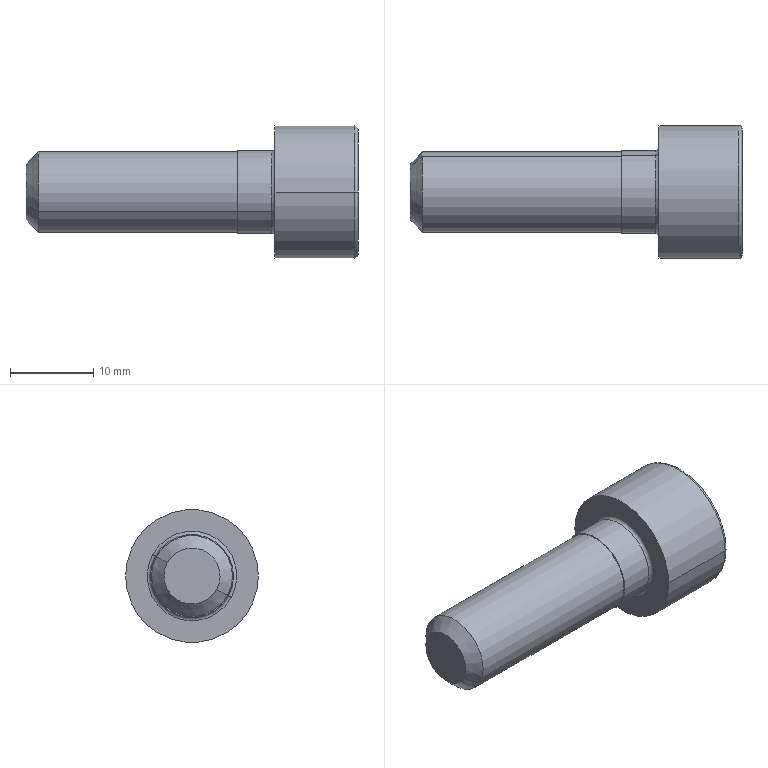Part | NX | features BREP 1 | 1 solid | 31 faces | box 40 x 16 x 16 mm | volume 3905 mm3 | cylinder 12 | plane 11 | torus 4 | cone 4 | commonest cylinder face diameters 9.149 x6 9.756 x2 10 x2 16 x2
STEP:
#1=CARTESIAN_POINT('',(0.,-8.,0.));
#2=VERTEX_POINT('',#1);
#3=CARTESIAN_POINT('',(0.,8.,0.));
#4=VERTEX_POINT('',#3);
#5=CARTESIAN_POINT('',(0.,0.,0.));
#6=DIRECTION('',(-1.,0.,0.));
#7=DIRECTION('',(0.,-1.,0.));
#8=AXIS2_PLACEMENT_3D('',#5,#6,#7);
#9=CIRCLE('',#8,8.);
#10=EDGE_CURVE('',#2,#4,#9,.T.);
#11=ORIENTED_EDGE('',*,*,#10,.F.);
#12=CARTESIAN_POINT('',(9.6,-8.,0.));
#13=VERTEX_POINT('',#12);
#14=CARTESIAN_POINT('',(9.6,-8.,0.));
#15=DIRECTION('',(-1.,0.,0.));
#16=VECTOR('',#15,1000.);
#17=LINE('',#14,#16);
#18=EDGE_CURVE('',#13,#2,#17,.T.);
#19=ORIENTED_EDGE('',*,*,#18,.F.);
#20=CARTESIAN_POINT('',(9.6,8.,0.));
#21=VERTEX_POINT('',#20);
#22=CARTESIAN_POINT('',(9.6,0.,0.));
#23=DIRECTION('',(1.,0.,0.));
#24=DIRECTION('',(0.,1.,0.));
#25=AXIS2_PLACEMENT_3D('',#22,#23,#24);
#26=CIRCLE('',#25,8.);
#27=EDGE_CURVE('',#21,#13,#26,.T.);
#28=ORIENTED_EDGE('',*,*,#27,.F.);
#29=CARTESIAN_POINT('',(9.6,8.,0.));
#30=DIRECTION('',(-1.,0.,0.));
#31=VECTOR('',#30,1000.);
#32=LINE('',#29,#31);
#33=EDGE_CURVE('',#21,#4,#32,.T.);
#34=ORIENTED_EDGE('',*,*,#33,.T.);
#35=EDGE_LOOP('',(#11,#19,#28,#34));
#36=FACE_BOUND('',#35,.T.);
#37=CARTESIAN_POINT('',(5.,0.,0.));
#38=DIRECTION('',(1.,0.,0.));
#39=DIRECTION('',(0.,1.,0.));
#40=AXIS2_PLACEMENT_3D('',#37,#38,#39);
#41=CYLINDRICAL_SURFACE('',#40,8.);
#42=ADVANCED_FACE('',(#36),#41,.T.);
#43=CARTESIAN_POINT('',(0.,0.,0.));
#44=DIRECTION('',(-1.,0.,0.));
#45=DIRECTION('',(0.,1.,0.));
#46=AXIS2_PLACEMENT_3D('',#43,#44,#45);
#47=CIRCLE('',#46,8.);
#48=EDGE_CURVE('',#4,#2,#47,.T.);
#49=ORIENTED_EDGE('',*,*,#48,.F.);
#50=ORIENTED_EDGE('',*,*,#33,.F.);
#51=CARTESIAN_POINT('',(9.6,0.,0.));
#52=DIRECTION('',(-1.,0.,0.));
#53=DIRECTION('',(0.,1.,0.));
#54=AXIS2_PLACEMENT_3D('',#51,#52,#53);
#55=CIRCLE('',#54,8.);
#56=EDGE_CURVE('',#21,#13,#55,.T.);
#57=ORIENTED_EDGE('',*,*,#56,.T.);
#58=ORIENTED_EDGE('',*,*,#18,.T.);
#59=EDGE_LOOP('',(#49,#50,#57,#58));
#60=FACE_BOUND('',#59,.T.);
#61=CARTESIAN_POINT('',(5.,0.,0.));
#62=DIRECTION('',(1.,0.,0.));
#63=DIRECTION('',(0.,1.,0.));
#64=AXIS2_PLACEMENT_3D('',#61,#62,#63);
#65=CYLINDRICAL_SURFACE('',#64,8.);
#66=ADVANCED_FACE('',(#60),#65,.T.);
#67=ORIENTED_EDGE('',*,*,#56,.F.);
#68=CARTESIAN_POINT('',(10.,7.6,0.));
#69=VERTEX_POINT('',#68);
#70=CARTESIAN_POINT('',(9.6,7.6,0.));
#71=DIRECTION('',(0.,0.,-1.));
#72=DIRECTION('',(0.,1.,0.));
#73=AXIS2_PLACEMENT_3D('',#70,#71,#72);
#74=CIRCLE('',#73,0.4);
#75=EDGE_CURVE('',#69,#21,#74,.F.);
#76=ORIENTED_EDGE('',*,*,#75,.F.);
#77=CARTESIAN_POINT('',(10.,-7.6,0.));
#78=VERTEX_POINT('',#77);
#79=CARTESIAN_POINT('',(10.,0.,0.));
#80=DIRECTION('',(1.,0.,0.));
#81=DIRECTION('',(0.,0.8749,-0.4843));
#82=AXIS2_PLACEMENT_3D('',#79,#80,#81);
#83=CIRCLE('',#82,7.6);
#84=EDGE_CURVE('',#78,#69,#83,.T.);
#85=ORIENTED_EDGE('',*,*,#84,.F.);
#86=CARTESIAN_POINT('',(9.6,-7.6,0.));
#87=DIRECTION('',(0.,0.,1.));
#88=DIRECTION('',(0.,-1.,0.));
#89=AXIS2_PLACEMENT_3D('',#86,#87,#88);
#90=CIRCLE('',#89,0.4);
#91=EDGE_CURVE('',#78,#13,#90,.F.);
#92=ORIENTED_EDGE('',*,*,#91,.T.);
#93=EDGE_LOOP('',(#67,#76,#85,#92));
#94=FACE_BOUND('',#93,.T.);
#95=CARTESIAN_POINT('',(9.6,0.,0.));
#96=DIRECTION('',(1.,0.,0.));
#97=DIRECTION('',(0.,-0.8749,0.4843));
#98=AXIS2_PLACEMENT_3D('',#95,#96,#97);
#99=TOROIDAL_SURFACE('',#98,7.6,0.4);
#100=ADVANCED_FACE('',(#94),#99,.T.);
#101=ORIENTED_EDGE('',*,*,#27,.T.);
#102=ORIENTED_EDGE('',*,*,#91,.F.);
#103=CARTESIAN_POINT('',(10.,0.,0.));
#104=DIRECTION('',(1.,0.,0.));
#105=DIRECTION('',(0.,1.,0.));
#106=AXIS2_PLACEMENT_3D('',#103,#104,#105);
#107=CIRCLE('',#106,7.6);
#108=EDGE_CURVE('',#69,#78,#107,.T.);
#109=ORIENTED_EDGE('',*,*,#108,.F.);
#110=ORIENTED_EDGE('',*,*,#75,.T.);
#111=EDGE_LOOP('',(#101,#102,#109,#110));
#112=FACE_BOUND('',#111,.T.);
#113=CARTESIAN_POINT('',(9.6,0.,0.));
#114=DIRECTION('',(1.,0.,0.));
#115=DIRECTION('',(0.,1.,0.));
#116=AXIS2_PLACEMENT_3D('',#113,#114,#115);
#117=TOROIDAL_SURFACE('',#116,7.6,0.4);
#118=ADVANCED_FACE('',(#112),#117,.T.);
#119=ORIENTED_EDGE('',*,*,#84,.T.);
#120=ORIENTED_EDGE('',*,*,#108,.T.);
#121=EDGE_LOOP('',(#119,#120));
#122=FACE_BOUND('',#121,.T.);
#123=CARTESIAN_POINT('',(10.,4.,-2.219));
#124=VERTEX_POINT('',#123);
#125=CARTESIAN_POINT('',(10.,3.922,-2.354));
#126=VERTEX_POINT('',#125);
#127=CARTESIAN_POINT('',(10.,0.,0.));
#128=DIRECTION('',(-1.,0.,0.));
#129=DIRECTION('',(0.,0.8744,-0.4852));
#130=AXIS2_PLACEMENT_3D('',#127,#128,#129);
#131=CIRCLE('',#130,4.574);
#132=EDGE_CURVE('',#124,#126,#131,.T.);
#133=ORIENTED_EDGE('',*,*,#132,.T.);
#134=CARTESIAN_POINT('',(10.,0.07788,-4.574));
#135=VERTEX_POINT('',#134);
#136=CARTESIAN_POINT('',(10.,3.922,-2.354));
#137=DIRECTION('',(0.,-0.866,-0.5));
#138=VECTOR('',#137,1000.);
#139=LINE('',#136,#138);
#140=EDGE_CURVE('',#126,#135,#139,.T.);
#141=ORIENTED_EDGE('',*,*,#140,.T.);
#142=CARTESIAN_POINT('',(10.,-0.07788,-4.574));
#143=VERTEX_POINT('',#142);
#144=CARTESIAN_POINT('',(10.,0.,0.));
#145=DIRECTION('',(1.,0.,0.));
#146=DIRECTION('',(0.,-0.01703,-0.9999));
#147=AXIS2_PLACEMENT_3D('',#144,#145,#146);
#148=CIRCLE('',#147,4.574);
#149=EDGE_CURVE('',#143,#135,#148,.T.);
#150=ORIENTED_EDGE('',*,*,#149,.F.);
#151=CARTESIAN_POINT('',(10.,-3.922,-2.354));
#152=VERTEX_POINT('',#151);
#153=CARTESIAN_POINT('',(10.,-0.07788,-4.574));
#154=DIRECTION('',(0.,-0.866,0.5));
#155=VECTOR('',#154,1000.);
#156=LINE('',#153,#155);
#157=EDGE_CURVE('',#143,#152,#156,.T.);
#158=ORIENTED_EDGE('',*,*,#157,.T.);
#159=CARTESIAN_POINT('',(10.,-4.,-2.219));
#160=VERTEX_POINT('',#159);
#161=CARTESIAN_POINT('',(10.,0.,0.));
#162=DIRECTION('',(-1.,0.,0.));
#163=DIRECTION('',(0.,-0.8574,-0.5147));
#164=AXIS2_PLACEMENT_3D('',#161,#162,#163);
#165=CIRCLE('',#164,4.574);
#166=EDGE_CURVE('',#152,#160,#165,.T.);
#167=ORIENTED_EDGE('',*,*,#166,.T.);
#168=CARTESIAN_POINT('',(10.,-4.,2.219));
#169=VERTEX_POINT('',#168);
#170=CARTESIAN_POINT('',(10.,-4.,-2.219));
#171=DIRECTION('',(0.,0.,1.));
#172=VECTOR('',#171,1000.);
#173=LINE('',#170,#172);
#174=EDGE_CURVE('',#160,#169,#173,.T.);
#175=ORIENTED_EDGE('',*,*,#174,.T.);
#176=CARTESIAN_POINT('',(10.,-3.922,2.354));
#177=VERTEX_POINT('',#176);
#178=CARTESIAN_POINT('',(10.,0.,0.));
#179=DIRECTION('',(-1.,0.,0.));
#180=DIRECTION('',(0.,-0.8744,0.4852));
#181=AXIS2_PLACEMENT_3D('',#178,#179,#180);
#182=CIRCLE('',#181,4.574);
#183=EDGE_CURVE('',#169,#177,#182,.T.);
#184=ORIENTED_EDGE('',*,*,#183,.T.);
#185=CARTESIAN_POINT('',(10.,-0.07788,4.574));
#186=VERTEX_POINT('',#185);
#187=CARTESIAN_POINT('',(10.,-3.922,2.354));
#188=DIRECTION('',(0.,0.866,0.5));
#189=VECTOR('',#188,1000.);
#190=LINE('',#187,#189);
#191=EDGE_CURVE('',#177,#186,#190,.T.);
#192=ORIENTED_EDGE('',*,*,#191,.T.);
#193=CARTESIAN_POINT('',(10.,0.07788,4.574));
#194=VERTEX_POINT('',#193);
#195=CARTESIAN_POINT('',(10.,0.,0.));
#196=DIRECTION('',(1.,0.,0.));
#197=DIRECTION('',(0.,0.01703,0.9999));
#198=AXIS2_PLACEMENT_3D('',#195,#196,#197);
#199=CIRCLE('',#198,4.574);
#200=EDGE_CURVE('',#194,#186,#199,.T.);
#201=ORIENTED_EDGE('',*,*,#200,.F.);
#202=CARTESIAN_POINT('',(10.,3.922,2.354));
#203=VERTEX_POINT('',#202);
#204=CARTESIAN_POINT('',(10.,0.07788,4.574));
#205=DIRECTION('',(0.,0.866,-0.5));
#206=VECTOR('',#205,1000.);
#207=LINE('',#204,#206);
#208=EDGE_CURVE('',#194,#203,#207,.T.);
#209=ORIENTED_EDGE('',*,*,#208,.T.);
#210=CARTESIAN_POINT('',(10.,4.,2.219));
#211=VERTEX_POINT('',#210);
#212=CARTESIAN_POINT('',(10.,0.,0.));
#213=DIRECTION('',(-1.,0.,0.));
#214=DIRECTION('',(0.,0.8574,0.5147));
#215=AXIS2_PLACEMENT_3D('',#212,#213,#214);
#216=CIRCLE('',#215,4.574);
#217=EDGE_CURVE('',#203,#211,#216,.T.);
#218=ORIENTED_EDGE('',*,*,#217,.T.);
#219=CARTESIAN_POINT('',(10.,4.,2.219));
#220=DIRECTION('',(0.,0.,-1.));
#221=VECTOR('',#220,1000.);
#222=LINE('',#219,#221);
#223=EDGE_CURVE('',#211,#124,#222,.T.);
#224=ORIENTED_EDGE('',*,*,#223,.T.);
#225=EDGE_LOOP('',(#133,#141,#150,#158,#167,#175,#184,#192,#201,#209,#218,#224));
#226=FACE_BOUND('',#225,.T.);
#227=CARTESIAN_POINT('',(10.,0.,0.));
#228=DIRECTION('',(1.,0.,0.));
#229=DIRECTION('',(0.,1.,0.));
#230=AXIS2_PLACEMENT_3D('',#227,#228,#229);
#231=PLANE('',#230);
#232=ADVANCED_FACE('',(#122,#226),#231,.T.);
#233=CARTESIAN_POINT('',(5.,4.,2.219));
#234=VERTEX_POINT('',#233);
#235=CARTESIAN_POINT('',(5.,4.,2.219));
#236=DIRECTION('',(1.,0.,0.));
#237=VECTOR('',#236,1000.);
#238=LINE('',#235,#237);
#239=EDGE_CURVE('',#234,#211,#238,.T.);
#240=ORIENTED_EDGE('',*,*,#239,.F.);
#241=CARTESIAN_POINT('',(5.,4.,-2.219));
#242=VERTEX_POINT('',#241);
#243=CARTESIAN_POINT('',(5.,4.,2.219));
#244=CARTESIAN_POINT('',(4.767,4.,1.389));
#245=CARTESIAN_POINT('',(4.569,4.,-0.0008489));
#246=CARTESIAN_POINT('',(4.767,4.,-1.388));
#247=CARTESIAN_POINT('',(5.,4.,-2.219));
#248=B_SPLINE_CURVE_WITH_KNOTS('',3,(#243,#244,#245,#246,#247),.UNSPECIFIED.,.F.,.F.,(4,1,4),(0.,0.5,1.),.UNSPECIFIED.);
#249=EDGE_CURVE('',#242,#234,#248,.F.);
#250=ORIENTED_EDGE('',*,*,#249,.F.);
#251=CARTESIAN_POINT('',(10.,4.,-2.219));
#252=DIRECTION('',(-1.,0.,0.));
#253=VECTOR('',#252,1000.);
#254=LINE('',#251,#253);
#255=EDGE_CURVE('',#124,#242,#254,.T.);
#256=ORIENTED_EDGE('',*,*,#255,.F.);
#257=ORIENTED_EDGE('',*,*,#223,.F.);
#258=EDGE_LOOP('',(#240,#250,#256,#257));
#259=FACE_BOUND('',#258,.T.);
#260=CARTESIAN_POINT('',(10.,4.,-2.309));
#261=DIRECTION('',(0.,-1.,0.));
#262=DIRECTION('',(0.,0.,-1.));
#263=AXIS2_PLACEMENT_3D('',#260,#261,#262);
#264=PLANE('',#263);
#265=ADVANCED_FACE('',(#259),#264,.T.);
#266=ORIENTED_EDGE('',*,*,#255,.T.);
#267=CARTESIAN_POINT('',(5.,3.922,-2.354));
#268=VERTEX_POINT('',#267);
#269=CARTESIAN_POINT('',(5.,0.,0.));
#270=DIRECTION('',(1.,0.,0.));
#271=DIRECTION('',(0.,0.8574,-0.5147));
#272=AXIS2_PLACEMENT_3D('',#269,#270,#271);
#273=CIRCLE('',#272,4.575);
#274=EDGE_CURVE('',#268,#242,#273,.T.);
#275=ORIENTED_EDGE('',*,*,#274,.F.);
#276=CARTESIAN_POINT('',(5.,3.922,-2.354));
#277=DIRECTION('',(1.,0.,0.));
#278=VECTOR('',#277,1000.);
#279=LINE('',#276,#278);
#280=EDGE_CURVE('',#268,#126,#279,.T.);
#281=ORIENTED_EDGE('',*,*,#280,.T.);
#282=ORIENTED_EDGE('',*,*,#132,.F.);
#283=EDGE_LOOP('',(#266,#275,#281,#282));
#284=FACE_BOUND('',#283,.T.);
#285=CARTESIAN_POINT('',(6.179,0.,0.));
#286=DIRECTION('',(-1.,0.,0.));
#287=DIRECTION('',(0.,0.4794,0.8776));
#288=AXIS2_PLACEMENT_3D('',#285,#286,#287);
#289=CYLINDRICAL_SURFACE('',#288,4.574);
#290=ADVANCED_FACE('',(#284),#289,.F.);
#291=ORIENTED_EDGE('',*,*,#280,.F.);
#292=CARTESIAN_POINT('',(5.,0.07788,-4.574));
#293=VERTEX_POINT('',#292);
#294=CARTESIAN_POINT('',(5.,3.922,-2.354));
#295=CARTESIAN_POINT('',(4.767,3.203,-2.769));
#296=CARTESIAN_POINT('',(4.569,1.999,-3.465));
#297=CARTESIAN_POINT('',(4.767,0.7977,-4.158));
#298=CARTESIAN_POINT('',(5.,0.07788,-4.574));
#299=B_SPLINE_CURVE_WITH_KNOTS('',3,(#294,#295,#296,#297,#298),.UNSPECIFIED.,.F.,.F.,(4,1,4),(0.,0.5,1.),.UNSPECIFIED.);
#300=EDGE_CURVE('',#293,#268,#299,.F.);
#301=ORIENTED_EDGE('',*,*,#300,.F.);
#302=CARTESIAN_POINT('',(10.,0.07788,-4.574));
#303=DIRECTION('',(-1.,0.000000087,0.00000005));
#304=VECTOR('',#303,1000.);
#305=LINE('',#302,#304);
#306=EDGE_CURVE('',#135,#293,#305,.T.);
#307=ORIENTED_EDGE('',*,*,#306,.F.);
#308=ORIENTED_EDGE('',*,*,#140,.F.);
#309=EDGE_LOOP('',(#291,#301,#307,#308));
#310=FACE_BOUND('',#309,.T.);
#311=CARTESIAN_POINT('',(10.,0.,-4.619));
#312=DIRECTION('',(0.,-0.5,0.866));
#313=DIRECTION('',(-1.,0.,0.));
#314=AXIS2_PLACEMENT_3D('',#311,#312,#313);
#315=PLANE('',#314);
#316=ADVANCED_FACE('',(#310),#315,.T.);
#317=CARTESIAN_POINT('',(5.,-0.07788,-4.574));
#318=VERTEX_POINT('',#317);
#319=CARTESIAN_POINT('',(5.,-0.07788,-4.574));
#320=DIRECTION('',(1.,0.000000043,-0.000000025));
#321=VECTOR('',#320,1000.);
#322=LINE('',#319,#321);
#323=EDGE_CURVE('',#318,#143,#322,.T.);
#324=ORIENTED_EDGE('',*,*,#323,.T.);
#325=ORIENTED_EDGE('',*,*,#149,.T.);
#326=ORIENTED_EDGE('',*,*,#306,.T.);
#327=CARTESIAN_POINT('',(5.,0.,0.));
#328=DIRECTION('',(1.,0.,0.));
#329=DIRECTION('',(0.,-0.01703,-0.9999));
#330=AXIS2_PLACEMENT_3D('',#327,#328,#329);
#331=CIRCLE('',#330,4.575);
#332=EDGE_CURVE('',#318,#293,#331,.T.);
#333=ORIENTED_EDGE('',*,*,#332,.F.);
#334=EDGE_LOOP('',(#324,#325,#326,#333));
#335=FACE_BOUND('',#334,.T.);
#336=CARTESIAN_POINT('',(6.179,0.,0.));
#337=DIRECTION('',(-1.,0.,0.));
#338=DIRECTION('',(0.,0.4794,0.8776));
#339=AXIS2_PLACEMENT_3D('',#336,#337,#338);
#340=CYLINDRICAL_SURFACE('',#339,4.574);
#341=ADVANCED_FACE('',(#335),#340,.F.);
#342=CARTESIAN_POINT('',(2.363,-0.003384,-0.00693));
#343=VERTEX_POINT('',#342);
#344=CARTESIAN_POINT('',(2.363,0.004101,0.006576));
#345=VERTEX_POINT('',#344);
#346=CARTESIAN_POINT('',(2.363,-0.003384,-0.00693));
#347=CARTESIAN_POINT('',(2.363,0.005447,-0.008722));
#348=CARTESIAN_POINT('',(2.363,0.01201,-0.001122));
#349=CARTESIAN_POINT('',(2.363,0.004101,0.006576));
#350=B_SPLINE_CURVE_WITH_KNOTS('',3,(#346,#347,#348,#349),.UNSPECIFIED.,.F.,.F.,(4,4),(0.,1.),.UNSPECIFIED.);
#351=EDGE_CURVE('',#343,#345,#350,.T.);
#352=ORIENTED_EDGE('',*,*,#351,.F.);
#353=CARTESIAN_POINT('',(4.669,-1.918,-3.511));
#354=VERTEX_POINT('',#353);
#355=CARTESIAN_POINT('',(4.669,-1.918,-3.511));
#356=CARTESIAN_POINT('',(4.413,-1.706,-3.123));
#357=CARTESIAN_POINT('',(4.074,-1.424,-2.608));
#358=CARTESIAN_POINT('',(3.773,-1.174,-2.149));
#359=CARTESIAN_POINT('',(3.61,-1.038,-1.901));
#360=CARTESIAN_POINT('',(3.541,-0.9811,-1.797));
#361=CARTESIAN_POINT('',(3.324,-0.8014,-1.468));
#362=CARTESIAN_POINT('',(3.181,-0.682,-1.249));
#363=CARTESIAN_POINT('',(3.036,-0.5621,-1.03));
#364=CARTESIAN_POINT('',(2.964,-0.5019,-0.9197));
#365=CARTESIAN_POINT('',(2.747,-0.3216,-0.5899));
#366=CARTESIAN_POINT('',(2.692,-0.2762,-0.5069));
#367=CARTESIAN_POINT('',(2.559,-0.1658,-0.3049));
#368=CARTESIAN_POINT('',(2.511,-0.1253,-0.2309));
#369=CARTESIAN_POINT('',(2.443,-0.06943,-0.1282));
#370=CARTESIAN_POINT('',(2.367,-0.006136,-0.01342));
#371=CARTESIAN_POINT('',(2.363,-0.003389,-0.006939));
#372=B_SPLINE_CURVE_WITH_KNOTS('',3,(#355,#356,#357,#358,#359,#360,#361,#362,#363,#364,#365,#366,#367,#368,#369,#370,#371),.UNSPECIFIED.,.F.,.F.,(4,1,1,1,1,1,1,1,1,1,1,1,1,1,4),(0.,0.25,0.375,0.4375,0.5,0.5625,0.625,0.6875,0.75,0.8125,0.875,0.9062,0.9375,0.9688,1.),.UNSPECIFIED.);
#373=EDGE_CURVE('',#343,#354,#372,.F.);
#374=ORIENTED_EDGE('',*,*,#373,.T.);
#375=CARTESIAN_POINT('',(5.,-0.07788,-4.574));
#376=CARTESIAN_POINT('',(4.787,-0.7349,-4.195));
#377=CARTESIAN_POINT('',(4.678,-1.33,-3.851));
#378=CARTESIAN_POINT('',(4.669,-1.918,-3.511));
#379=B_SPLINE_CURVE_WITH_KNOTS('',3,(#375,#376,#377,#378),.UNSPECIFIED.,.F.,.F.,(4,4),(0.,1.),.UNSPECIFIED.);
#380=EDGE_CURVE('',#354,#318,#379,.F.);
#381=ORIENTED_EDGE('',*,*,#380,.T.);
#382=ORIENTED_EDGE('',*,*,#332,.T.);
#383=ORIENTED_EDGE('',*,*,#300,.T.);
#384=ORIENTED_EDGE('',*,*,#274,.T.);
#385=ORIENTED_EDGE('',*,*,#249,.T.);
#386=CARTESIAN_POINT('',(5.,3.922,2.354));
#387=VERTEX_POINT('',#386);
#388=CARTESIAN_POINT('',(5.,0.,0.));
#389=DIRECTION('',(1.,0.,0.));
#390=DIRECTION('',(0.,0.8744,0.4852));
#391=AXIS2_PLACEMENT_3D('',#388,#389,#390);
#392=CIRCLE('',#391,4.575);
#393=EDGE_CURVE('',#234,#387,#392,.T.);
#394=ORIENTED_EDGE('',*,*,#393,.T.);
#395=CARTESIAN_POINT('',(4.669,1.918,3.511));
#396=VERTEX_POINT('',#395);
#397=CARTESIAN_POINT('',(4.669,1.918,3.511));
#398=CARTESIAN_POINT('',(4.659,2.568,3.136));
#399=CARTESIAN_POINT('',(4.77,3.212,2.764));
#400=CARTESIAN_POINT('',(5.,3.922,2.354));
#401=B_SPLINE_CURVE_WITH_KNOTS('',3,(#397,#398,#399,#400),.UNSPECIFIED.,.F.,.F.,(4,4),(0.,1.),.UNSPECIFIED.);
#402=EDGE_CURVE('',#387,#396,#401,.F.);
#403=ORIENTED_EDGE('',*,*,#402,.T.);
#404=CARTESIAN_POINT('',(4.669,1.918,3.511));
#405=CARTESIAN_POINT('',(4.413,1.706,3.123));
#406=CARTESIAN_POINT('',(4.074,1.425,2.608));
#407=CARTESIAN_POINT('',(3.773,1.174,2.149));
#408=CARTESIAN_POINT('',(3.61,1.039,1.901));
#409=CARTESIAN_POINT('',(3.541,0.9815,1.796));
#410=CARTESIAN_POINT('',(3.325,0.8021,1.468));
#411=CARTESIAN_POINT('',(3.181,0.6827,1.249));
#412=CARTESIAN_POINT('',(3.036,0.5629,1.03));
#413=CARTESIAN_POINT('',(2.964,0.5026,0.9193));
#414=CARTESIAN_POINT('',(2.747,0.3226,0.5897));
#415=CARTESIAN_POINT('',(2.692,0.2771,0.5064));
#416=CARTESIAN_POINT('',(2.559,0.1669,0.3046));
#417=CARTESIAN_POINT('',(2.51,0.1262,0.2301));
#418=CARTESIAN_POINT('',(2.444,0.07082,0.1287));
#419=CARTESIAN_POINT('',(2.366,0.006312,0.01062));
#420=CARTESIAN_POINT('',(2.363,0.004105,0.006581));
#421=B_SPLINE_CURVE_WITH_KNOTS('',3,(#404,#405,#406,#407,#408,#409,#410,#411,#412,#413,#414,#415,#416,#417,#418,#419,#420),.UNSPECIFIED.,.F.,.F.,(4,1,1,1,1,1,1,1,1,1,1,1,1,1,4),(0.,0.25,0.375,0.4375,0.5,0.5625,0.625,0.6875,0.75,0.8125,0.875,0.9062,0.9375,0.9688,1.),.UNSPECIFIED.);
#422=EDGE_CURVE('',#396,#345,#421,.T.);
#423=ORIENTED_EDGE('',*,*,#422,.T.);
#424=EDGE_LOOP('',(#352,#374,#381,#382,#383,#384,#385,#394,#403,#423));
#425=FACE_BOUND('',#424,.T.);
#426=CARTESIAN_POINT('',(3.707,0.,0.));
#427=DIRECTION('',(1.,0.,0.));
#428=DIRECTION('',(0.,0.4794,0.8776));
#429=AXIS2_PLACEMENT_3D('',#426,#427,#428);
#430=CONICAL_SURFACE('',#429,2.335,1.047);
#431=ADVANCED_FACE('',(#425),#430,.F.);
#432=ORIENTED_EDGE('',*,*,#373,.F.);
#433=CARTESIAN_POINT('',(2.363,-0.007776,0.));
#434=VERTEX_POINT('',#433);
#435=CARTESIAN_POINT('',(2.363,-0.007776,0.));
#436=CARTESIAN_POINT('',(2.363,-0.007394,-0.003114));
#437=CARTESIAN_POINT('',(2.363,-0.00593,-0.005424));
#438=CARTESIAN_POINT('',(2.363,-0.003384,-0.00693));
#439=B_SPLINE_CURVE_WITH_KNOTS('',3,(#435,#436,#437,#438),.UNSPECIFIED.,.F.,.F.,(4,4),(0.,1.),.UNSPECIFIED.);
#440=EDGE_CURVE('',#434,#343,#439,.T.);
#441=ORIENTED_EDGE('',*,*,#440,.F.);
#442=CARTESIAN_POINT('',(2.363,0.004101,0.006576));
#443=CARTESIAN_POINT('',(2.363,-0.001035,0.008767));
#444=CARTESIAN_POINT('',(2.363,-0.0067,0.007369));
#445=CARTESIAN_POINT('',(2.363,-0.007776,0.));
#446=B_SPLINE_CURVE_WITH_KNOTS('',3,(#442,#443,#444,#445),.UNSPECIFIED.,.F.,.F.,(4,4),(0.,1.),.UNSPECIFIED.);
#447=EDGE_CURVE('',#345,#434,#446,.T.);
#448=ORIENTED_EDGE('',*,*,#447,.F.);
#449=ORIENTED_EDGE('',*,*,#422,.F.);
#450=CARTESIAN_POINT('',(5.,0.07788,4.574));
#451=VERTEX_POINT('',#450);
#452=CARTESIAN_POINT('',(5.,0.07788,4.574));
#453=CARTESIAN_POINT('',(4.792,0.7218,4.202));
#454=CARTESIAN_POINT('',(4.678,1.319,3.858));
#455=CARTESIAN_POINT('',(4.669,1.918,3.511));
#456=B_SPLINE_CURVE_WITH_KNOTS('',3,(#452,#453,#454,#455),.UNSPECIFIED.,.F.,.F.,(4,4),(0.,1.),.UNSPECIFIED.);
#457=EDGE_CURVE('',#451,#396,#456,.T.);
#458=ORIENTED_EDGE('',*,*,#457,.F.);
#459=CARTESIAN_POINT('',(5.,-0.07788,4.574));
#460=VERTEX_POINT('',#459);
#461=CARTESIAN_POINT('',(5.,0.,0.));
#462=DIRECTION('',(1.,0.,0.));
#463=DIRECTION('',(0.,0.01703,0.9999));
#464=AXIS2_PLACEMENT_3D('',#461,#462,#463);
#465=CIRCLE('',#464,4.575);
#466=EDGE_CURVE('',#451,#460,#465,.T.);
#467=ORIENTED_EDGE('',*,*,#466,.T.);
#468=CARTESIAN_POINT('',(5.,-3.922,2.354));
#469=VERTEX_POINT('',#468);
#470=CARTESIAN_POINT('',(5.,-3.922,2.354));
#471=CARTESIAN_POINT('',(4.538,-2.493,3.179));
#472=CARTESIAN_POINT('',(4.537,-1.509,3.748));
#473=CARTESIAN_POINT('',(5.,-0.07788,4.574));
#474=B_SPLINE_CURVE_WITH_KNOTS('',3,(#470,#471,#472,#473),.UNSPECIFIED.,.F.,.F.,(4,4),(0.,1.),.UNSPECIFIED.);
#475=EDGE_CURVE('',#460,#469,#474,.F.);
#476=ORIENTED_EDGE('',*,*,#475,.T.);
#477=CARTESIAN_POINT('',(5.,-4.,2.219));
#478=VERTEX_POINT('',#477);
#479=CARTESIAN_POINT('',(5.,0.,0.));
#480=DIRECTION('',(1.,0.,0.));
#481=DIRECTION('',(0.,-0.8574,0.5147));
#482=AXIS2_PLACEMENT_3D('',#479,#480,#481);
#483=CIRCLE('',#482,4.575);
#484=EDGE_CURVE('',#469,#478,#483,.T.);
#485=ORIENTED_EDGE('',*,*,#484,.T.);
#486=CARTESIAN_POINT('',(5.,-4.,-2.219));
#487=VERTEX_POINT('',#486);
#488=CARTESIAN_POINT('',(5.,-4.,-2.219));
#489=CARTESIAN_POINT('',(4.767,-4.,-1.389));
#490=CARTESIAN_POINT('',(4.569,-4.,0.0008489));
#491=CARTESIAN_POINT('',(4.767,-4.,1.388));
#492=CARTESIAN_POINT('',(5.,-4.,2.219));
#493=B_SPLINE_CURVE_WITH_KNOTS('',3,(#488,#489,#490,#491,#492),.UNSPECIFIED.,.F.,.F.,(4,1,4),(0.,0.5,1.),.UNSPECIFIED.);
#494=EDGE_CURVE('',#478,#487,#493,.F.);
#495=ORIENTED_EDGE('',*,*,#494,.T.);
#496=CARTESIAN_POINT('',(5.,-3.922,-2.354));
#497=VERTEX_POINT('',#496);
#498=CARTESIAN_POINT('',(5.,0.,0.));
#499=DIRECTION('',(1.,0.,0.));
#500=DIRECTION('',(0.,-0.8744,-0.4852));
#501=AXIS2_PLACEMENT_3D('',#498,#499,#500);
#502=CIRCLE('',#501,4.575);
#503=EDGE_CURVE('',#487,#497,#502,.T.);
#504=ORIENTED_EDGE('',*,*,#503,.T.);
#505=CARTESIAN_POINT('',(4.669,-1.918,-3.511));
#506=CARTESIAN_POINT('',(4.659,-2.56,-3.141));
#507=CARTESIAN_POINT('',(4.767,-3.203,-2.77));
#508=CARTESIAN_POINT('',(5.,-3.922,-2.354));
#509=B_SPLINE_CURVE_WITH_KNOTS('',3,(#505,#506,#507,#508),.UNSPECIFIED.,.F.,.F.,(4,4),(0.,1.),.UNSPECIFIED.);
#510=EDGE_CURVE('',#497,#354,#509,.F.);
#511=ORIENTED_EDGE('',*,*,#510,.T.);
#512=EDGE_LOOP('',(#432,#441,#448,#449,#458,#467,#476,#485,#495,#504,#511));
#513=FACE_BOUND('',#512,.T.);
#514=CARTESIAN_POINT('',(3.707,0.,0.));
#515=DIRECTION('',(1.,0.,0.));
#516=DIRECTION('',(0.,0.4794,0.8776));
#517=AXIS2_PLACEMENT_3D('',#514,#515,#516);
#518=CONICAL_SURFACE('',#517,2.335,1.047);
#519=ADVANCED_FACE('',(#513),#518,.F.);
#520=ORIENTED_EDGE('',*,*,#323,.F.);
#521=ORIENTED_EDGE('',*,*,#380,.F.);
#522=ORIENTED_EDGE('',*,*,#510,.F.);
#523=CARTESIAN_POINT('',(10.,-3.922,-2.354));
#524=DIRECTION('',(-1.,0.,0.));
#525=VECTOR('',#524,1000.);
#526=LINE('',#523,#525);
#527=EDGE_CURVE('',#152,#497,#526,.T.);
#528=ORIENTED_EDGE('',*,*,#527,.F.);
#529=ORIENTED_EDGE('',*,*,#157,.F.);
#530=EDGE_LOOP('',(#520,#521,#522,#528,#529));
#531=FACE_BOUND('',#530,.T.);
#532=CARTESIAN_POINT('',(10.,-4.,-2.309));
#533=DIRECTION('',(0.,0.5,0.866));
#534=DIRECTION('',(1.,0.,0.));
#535=AXIS2_PLACEMENT_3D('',#532,#533,#534);
#536=PLANE('',#535);
#537=ADVANCED_FACE('',(#531),#536,.T.);
#538=ORIENTED_EDGE('',*,*,#503,.F.);
#539=CARTESIAN_POINT('',(5.,-4.,-2.219));
#540=DIRECTION('',(1.,0.,0.));
#541=VECTOR('',#540,1000.);
#542=LINE('',#539,#541);
#543=EDGE_CURVE('',#487,#160,#542,.T.);
#544=ORIENTED_EDGE('',*,*,#543,.T.);
#545=ORIENTED_EDGE('',*,*,#166,.F.);
#546=ORIENTED_EDGE('',*,*,#527,.T.);
#547=EDGE_LOOP('',(#538,#544,#545,#546));
#548=FACE_BOUND('',#547,.T.);
#549=CARTESIAN_POINT('',(6.179,0.,0.));
#550=DIRECTION('',(-1.,0.,0.));
#551=DIRECTION('',(0.,0.4794,0.8776));
#552=AXIS2_PLACEMENT_3D('',#549,#550,#551);
#553=CYLINDRICAL_SURFACE('',#552,4.574);
#554=ADVANCED_FACE('',(#548),#553,.F.);
#555=ORIENTED_EDGE('',*,*,#543,.F.);
#556=ORIENTED_EDGE('',*,*,#494,.F.);
#557=CARTESIAN_POINT('',(10.,-4.,2.219));
#558=DIRECTION('',(-1.,0.,0.));
#559=VECTOR('',#558,1000.);
#560=LINE('',#557,#559);
#561=EDGE_CURVE('',#169,#478,#560,.T.);
#562=ORIENTED_EDGE('',*,*,#561,.F.);
#563=ORIENTED_EDGE('',*,*,#174,.F.);
#564=EDGE_LOOP('',(#555,#556,#562,#563));
#565=FACE_BOUND('',#564,.T.);
#566=CARTESIAN_POINT('',(10.,-4.,2.309));
#567=DIRECTION('',(0.,1.,0.));
#568=DIRECTION('',(1.,0.,0.));
#569=AXIS2_PLACEMENT_3D('',#566,#567,#568);
#570=PLANE('',#569);
#571=ADVANCED_FACE('',(#565),#570,.T.);
#572=ORIENTED_EDGE('',*,*,#561,.T.);
#573=ORIENTED_EDGE('',*,*,#484,.F.);
#574=CARTESIAN_POINT('',(5.,-3.922,2.354));
#575=DIRECTION('',(1.,0.,0.));
#576=VECTOR('',#575,1000.);
#577=LINE('',#574,#576);
#578=EDGE_CURVE('',#469,#177,#577,.T.);
#579=ORIENTED_EDGE('',*,*,#578,.T.);
#580=ORIENTED_EDGE('',*,*,#183,.F.);
#581=EDGE_LOOP('',(#572,#573,#579,#580));
#582=FACE_BOUND('',#581,.T.);
#583=CARTESIAN_POINT('',(6.179,0.,0.));
#584=DIRECTION('',(-1.,0.,0.));
#585=DIRECTION('',(0.,0.4794,0.8776));
#586=AXIS2_PLACEMENT_3D('',#583,#584,#585);
#587=CYLINDRICAL_SURFACE('',#586,4.574);
#588=ADVANCED_FACE('',(#582),#587,.F.);
#589=ORIENTED_EDGE('',*,*,#578,.F.);
#590=ORIENTED_EDGE('',*,*,#475,.F.);
#591=CARTESIAN_POINT('',(10.,-0.07788,4.574));
#592=DIRECTION('',(-1.,-0.000000087,-0.00000005));
#593=VECTOR('',#592,1000.);
#594=LINE('',#591,#593);
#595=EDGE_CURVE('',#186,#460,#594,.T.);
#596=ORIENTED_EDGE('',*,*,#595,.F.);
#597=ORIENTED_EDGE('',*,*,#191,.F.);
#598=EDGE_LOOP('',(#589,#590,#596,#597));
#599=FACE_BOUND('',#598,.T.);
#600=CARTESIAN_POINT('',(10.,0.,4.619));
#601=DIRECTION('',(0.,0.5,-0.866));
#602=DIRECTION('',(-1.,0.,0.));
#603=AXIS2_PLACEMENT_3D('',#600,#601,#602);
#604=PLANE('',#603);
#605=ADVANCED_FACE('',(#599),#604,.T.);
#606=CARTESIAN_POINT('',(5.,0.07788,4.574));
#607=DIRECTION('',(1.,-0.000000043,0.000000025));
#608=VECTOR('',#607,1000.);
#609=LINE('',#606,#608);
#610=EDGE_CURVE('',#451,#194,#609,.T.);
#611=ORIENTED_EDGE('',*,*,#610,.T.);
#612=ORIENTED_EDGE('',*,*,#200,.T.);
#613=ORIENTED_EDGE('',*,*,#595,.T.);
#614=ORIENTED_EDGE('',*,*,#466,.F.);
#615=EDGE_LOOP('',(#611,#612,#613,#614));
#616=FACE_BOUND('',#615,.T.);
#617=CARTESIAN_POINT('',(6.179,0.,0.));
#618=DIRECTION('',(-1.,0.,0.));
#619=DIRECTION('',(0.,0.4794,0.8776));
#620=AXIS2_PLACEMENT_3D('',#617,#618,#619);
#621=CYLINDRICAL_SURFACE('',#620,4.574);
#622=ADVANCED_FACE('',(#616),#621,.F.);
#623=ORIENTED_EDGE('',*,*,#610,.F.);
#624=ORIENTED_EDGE('',*,*,#457,.T.);
#625=ORIENTED_EDGE('',*,*,#402,.F.);
#626=CARTESIAN_POINT('',(10.,3.922,2.354));
#627=DIRECTION('',(-1.,0.,0.));
#628=VECTOR('',#627,1000.);
#629=LINE('',#626,#628);
#630=EDGE_CURVE('',#203,#387,#629,.T.);
#631=ORIENTED_EDGE('',*,*,#630,.F.);
#632=ORIENTED_EDGE('',*,*,#208,.F.);
#633=EDGE_LOOP('',(#623,#624,#625,#631,#632));
#634=FACE_BOUND('',#633,.T.);
#635=CARTESIAN_POINT('',(10.,4.,2.309));
#636=DIRECTION('',(0.,-0.5,-0.866));
#637=DIRECTION('',(0.,-0.866,0.5));
#638=AXIS2_PLACEMENT_3D('',#635,#636,#637);
#639=PLANE('',#638);
#640=ADVANCED_FACE('',(#634),#639,.T.);
#641=ORIENTED_EDGE('',*,*,#393,.F.);
#642=ORIENTED_EDGE('',*,*,#239,.T.);
#643=ORIENTED_EDGE('',*,*,#217,.F.);
#644=ORIENTED_EDGE('',*,*,#630,.T.);
#645=EDGE_LOOP('',(#641,#642,#643,#644));
#646=FACE_BOUND('',#645,.T.);
#647=CARTESIAN_POINT('',(6.179,0.,0.));
#648=DIRECTION('',(-1.,0.,0.));
#649=DIRECTION('',(0.,0.4794,0.8776));
#650=AXIS2_PLACEMENT_3D('',#647,#648,#649);
#651=CYLINDRICAL_SURFACE('',#650,4.574);
#652=ADVANCED_FACE('',(#646),#651,.F.);
#653=ORIENTED_EDGE('',*,*,#440,.T.);
#654=ORIENTED_EDGE('',*,*,#351,.T.);
#655=ORIENTED_EDGE('',*,*,#447,.T.);
#656=EDGE_LOOP('',(#653,#654,#655));
#657=FACE_BOUND('',#656,.T.);
#658=CARTESIAN_POINT('',(2.363,0.,0.));
#659=DIRECTION('',(1.,0.,0.));
#660=DIRECTION('',(0.,1.,0.));
#661=AXIS2_PLACEMENT_3D('',#658,#659,#660);
#662=PLANE('',#661);
#663=ADVANCED_FACE('',(#657),#662,.T.);
#664=ORIENTED_EDGE('',*,*,#10,.T.);
#665=ORIENTED_EDGE('',*,*,#48,.T.);
#666=EDGE_LOOP('',(#664,#665));
#667=FACE_BOUND('',#666,.T.);
#668=CARTESIAN_POINT('',(0.,-4.739,-2.589));
#669=VERTEX_POINT('',#668);
#670=CARTESIAN_POINT('',(0.,4.739,2.589));
#671=VERTEX_POINT('',#670);
#672=CARTESIAN_POINT('',(0.,0.,0.));
#673=DIRECTION('',(1.,0.,0.));
#674=DIRECTION('',(0.,0.9996,0.02657));
#675=AXIS2_PLACEMENT_3D('',#672,#673,#674);
#676=CIRCLE('',#675,5.4);
#677=EDGE_CURVE('',#669,#671,#676,.T.);
#678=ORIENTED_EDGE('',*,*,#677,.T.);
#679=CARTESIAN_POINT('',(0.,0.,0.));
#680=DIRECTION('',(1.,0.,0.));
#681=DIRECTION('',(0.,0.8776,0.4794));
#682=AXIS2_PLACEMENT_3D('',#679,#680,#681);
#683=CIRCLE('',#682,5.4);
#684=EDGE_CURVE('',#671,#669,#683,.T.);
#685=ORIENTED_EDGE('',*,*,#684,.T.);
#686=EDGE_LOOP('',(#678,#685));
#687=FACE_BOUND('',#686,.T.);
#688=CARTESIAN_POINT('',(0.,0.,0.));
#689=DIRECTION('',(1.,0.,0.));
#690=DIRECTION('',(0.,1.,0.));
#691=AXIS2_PLACEMENT_3D('',#688,#689,#690);
#692=PLANE('',#691);
#693=ADVANCED_FACE('',(#667,#687),#692,.F.);
#694=ORIENTED_EDGE('',*,*,#677,.F.);
#695=CARTESIAN_POINT('',(-0.4,-4.388,-2.397));
#696=VERTEX_POINT('',#695);
#697=CARTESIAN_POINT('',(-0.4,-4.739,-2.589));
#698=DIRECTION('',(0.,0.4794,-0.8776));
#699=DIRECTION('',(0.,0.8776,0.4794));
#700=AXIS2_PLACEMENT_3D('',#697,#698,#699);
#701=CIRCLE('',#700,0.4);
#702=EDGE_CURVE('',#696,#669,#701,.T.);
#703=ORIENTED_EDGE('',*,*,#702,.F.);
#704=CARTESIAN_POINT('',(-0.4,4.388,2.397));
#705=VERTEX_POINT('',#704);
#706=CARTESIAN_POINT('',(-0.4,0.,0.));
#707=DIRECTION('',(1.,0.,0.));
#708=DIRECTION('',(0.,-0.8776,-0.4794));
#709=AXIS2_PLACEMENT_3D('',#706,#707,#708);
#710=CIRCLE('',#709,5.);
#711=EDGE_CURVE('',#696,#705,#710,.T.);
#712=ORIENTED_EDGE('',*,*,#711,.T.);
#713=CARTESIAN_POINT('',(-0.4,4.739,2.589));
#714=DIRECTION('',(0.,-0.4794,0.8776));
#715=DIRECTION('',(0.,-0.8776,-0.4794));
#716=AXIS2_PLACEMENT_3D('',#713,#714,#715);
#717=CIRCLE('',#716,0.4);
#718=EDGE_CURVE('',#705,#671,#717,.T.);
#719=ORIENTED_EDGE('',*,*,#718,.T.);
#720=EDGE_LOOP('',(#694,#703,#712,#719));
#721=FACE_BOUND('',#720,.T.);
#722=CARTESIAN_POINT('',(-0.4,0.,0.));
#723=DIRECTION('',(1.,0.,0.));
#724=DIRECTION('',(0.,-0.9996,-0.02657));
#725=AXIS2_PLACEMENT_3D('',#722,#723,#724);
#726=TOROIDAL_SURFACE('',#725,5.4,0.4);
#727=ADVANCED_FACE('',(#721),#726,.F.);
#728=ORIENTED_EDGE('',*,*,#718,.F.);
#729=CARTESIAN_POINT('',(-0.4,0.,0.));
#730=DIRECTION('',(1.,0.,0.));
#731=DIRECTION('',(0.,0.8776,0.4794));
#732=AXIS2_PLACEMENT_3D('',#729,#730,#731);
#733=CIRCLE('',#732,5.);
#734=EDGE_CURVE('',#705,#696,#733,.T.);
#735=ORIENTED_EDGE('',*,*,#734,.T.);
#736=ORIENTED_EDGE('',*,*,#702,.T.);
#737=ORIENTED_EDGE('',*,*,#684,.F.);
#738=EDGE_LOOP('',(#728,#735,#736,#737));
#739=FACE_BOUND('',#738,.T.);
#740=CARTESIAN_POINT('',(-0.4,0.,0.));
#741=DIRECTION('',(1.,0.,0.));
#742=DIRECTION('',(0.,0.8776,0.4794));
#743=AXIS2_PLACEMENT_3D('',#740,#741,#742);
#744=TOROIDAL_SURFACE('',#743,5.4,0.4);
#745=ADVANCED_FACE('',(#739),#744,.F.);
#746=CARTESIAN_POINT('',(-4.5,-4.388,-2.397));
#747=VERTEX_POINT('',#746);
#748=CARTESIAN_POINT('',(-4.5,4.388,2.397));
#749=VERTEX_POINT('',#748);
#750=CARTESIAN_POINT('',(-4.5,0.,0.));
#751=DIRECTION('',(-1.,0.,0.));
#752=DIRECTION('',(0.,-0.8776,-0.4794));
#753=AXIS2_PLACEMENT_3D('',#750,#751,#752);
#754=CIRCLE('',#753,5.);
#755=EDGE_CURVE('',#747,#749,#754,.T.);
#756=ORIENTED_EDGE('',*,*,#755,.F.);
#757=CARTESIAN_POINT('',(-4.5,-4.388,-2.397));
#758=DIRECTION('',(1.,0.,0.));
#759=VECTOR('',#758,1000.);
#760=LINE('',#757,#759);
#761=EDGE_CURVE('',#747,#696,#760,.T.);
#762=ORIENTED_EDGE('',*,*,#761,.T.);
#763=ORIENTED_EDGE('',*,*,#734,.F.);
#764=CARTESIAN_POINT('',(-4.5,4.388,2.397));
#765=DIRECTION('',(1.,0.,0.));
#766=VECTOR('',#765,1000.);
#767=LINE('',#764,#766);
#768=EDGE_CURVE('',#749,#705,#767,.T.);
#769=ORIENTED_EDGE('',*,*,#768,.F.);
#770=EDGE_LOOP('',(#756,#762,#763,#769));
#771=FACE_BOUND('',#770,.T.);
#772=CARTESIAN_POINT('',(-15.,0.,0.));
#773=DIRECTION('',(1.,0.,0.));
#774=DIRECTION('',(0.,0.8776,0.4794));
#775=AXIS2_PLACEMENT_3D('',#772,#773,#774);
#776=CYLINDRICAL_SURFACE('',#775,5.);
#777=ADVANCED_FACE('',(#771),#776,.T.);
#778=CARTESIAN_POINT('',(-4.5,0.,0.));
#779=DIRECTION('',(-1.,0.,0.));
#780=DIRECTION('',(0.,0.8776,0.4794));
#781=AXIS2_PLACEMENT_3D('',#778,#779,#780);
#782=CIRCLE('',#781,5.);
#783=EDGE_CURVE('',#749,#747,#782,.T.);
#784=ORIENTED_EDGE('',*,*,#783,.F.);
#785=ORIENTED_EDGE('',*,*,#768,.T.);
#786=ORIENTED_EDGE('',*,*,#711,.F.);
#787=ORIENTED_EDGE('',*,*,#761,.F.);
#788=EDGE_LOOP('',(#784,#785,#786,#787));
#789=FACE_BOUND('',#788,.T.);
#790=CARTESIAN_POINT('',(-15.,0.,0.));
#791=DIRECTION('',(1.,0.,0.));
#792=DIRECTION('',(0.,0.8776,0.4794));
#793=AXIS2_PLACEMENT_3D('',#790,#791,#792);
#794=CYLINDRICAL_SURFACE('',#793,5.);
#795=ADVANCED_FACE('',(#789),#794,.T.);
#796=ORIENTED_EDGE('',*,*,#783,.T.);
#797=ORIENTED_EDGE('',*,*,#755,.T.);
#798=EDGE_LOOP('',(#796,#797));
#799=FACE_BOUND('',#798,.T.);
#800=CARTESIAN_POINT('',(-4.5,4.281,2.339));
#801=VERTEX_POINT('',#800);
#802=CARTESIAN_POINT('',(-4.5,-4.281,-2.339));
#803=VERTEX_POINT('',#802);
#804=CARTESIAN_POINT('',(-4.5,0.,0.));
#805=DIRECTION('',(1.,0.,0.));
#806=DIRECTION('',(0.,0.8776,0.4794));
#807=AXIS2_PLACEMENT_3D('',#804,#805,#806);
#808=CIRCLE('',#807,4.878);
#809=EDGE_CURVE('',#801,#803,#808,.T.);
#810=ORIENTED_EDGE('',*,*,#809,.T.);
#811=CARTESIAN_POINT('',(-4.5,0.,0.));
#812=DIRECTION('',(1.,0.,0.));
#813=DIRECTION('',(0.,-0.8776,-0.4794));
#814=AXIS2_PLACEMENT_3D('',#811,#812,#813);
#815=CIRCLE('',#814,4.878);
#816=EDGE_CURVE('',#803,#801,#815,.T.);
#817=ORIENTED_EDGE('',*,*,#816,.T.);
#818=EDGE_LOOP('',(#810,#817));
#819=FACE_BOUND('',#818,.T.);
#820=CARTESIAN_POINT('',(-4.5,5.,0.));
#821=DIRECTION('',(1.,0.,0.));
#822=DIRECTION('',(0.,1.,0.));
#823=AXIS2_PLACEMENT_3D('',#820,#821,#822);
#824=PLANE('',#823);
#825=ADVANCED_FACE('',(#799,#819),#824,.F.);
#826=ORIENTED_EDGE('',*,*,#816,.F.);
#827=CARTESIAN_POINT('',(-28.5,-4.281,-2.339));
#828=VERTEX_POINT('',#827);
#829=CARTESIAN_POINT('',(-28.5,-4.281,-2.339));
#830=DIRECTION('',(1.,0.,0.));
#831=VECTOR('',#830,1000.);
#832=LINE('',#829,#831);
#833=EDGE_CURVE('',#803,#828,#832,.F.);
#834=ORIENTED_EDGE('',*,*,#833,.T.);
#835=CARTESIAN_POINT('',(-28.5,4.281,2.339));
#836=VERTEX_POINT('',#835);
#837=CARTESIAN_POINT('',(-28.5,0.,0.));
#838=DIRECTION('',(-1.,0.,0.));
#839=DIRECTION('',(0.,0.9918,-0.128));
#840=AXIS2_PLACEMENT_3D('',#837,#838,#839);
#841=CIRCLE('',#840,4.878);
#842=EDGE_CURVE('',#836,#828,#841,.T.);
#843=ORIENTED_EDGE('',*,*,#842,.F.);
#844=CARTESIAN_POINT('',(-28.5,4.281,2.339));
#845=DIRECTION('',(1.,0.,0.));
#846=VECTOR('',#845,1000.);
#847=LINE('',#844,#846);
#848=EDGE_CURVE('',#801,#836,#847,.F.);
#849=ORIENTED_EDGE('',*,*,#848,.F.);
#850=EDGE_LOOP('',(#826,#834,#843,#849));
#851=FACE_BOUND('',#850,.T.);
#852=CARTESIAN_POINT('',(-15.,0.,0.));
#853=DIRECTION('',(1.,0.,0.));
#854=DIRECTION('',(0.,0.8776,0.4794));
#855=AXIS2_PLACEMENT_3D('',#852,#853,#854);
#856=CYLINDRICAL_SURFACE('',#855,4.878);
#857=ADVANCED_FACE('',(#851),#856,.T.);
#858=ORIENTED_EDGE('',*,*,#833,.F.);
#859=ORIENTED_EDGE('',*,*,#809,.F.);
#860=ORIENTED_EDGE('',*,*,#848,.T.);
#861=CARTESIAN_POINT('',(-28.5,0.,0.));
#862=DIRECTION('',(-1.,0.,0.));
#863=DIRECTION('',(0.,-0.8776,-0.4794));
#864=AXIS2_PLACEMENT_3D('',#861,#862,#863);
#865=CIRCLE('',#864,4.878);
#866=EDGE_CURVE('',#828,#836,#865,.T.);
#867=ORIENTED_EDGE('',*,*,#866,.F.);
#868=EDGE_LOOP('',(#858,#859,#860,#867));
#869=FACE_BOUND('',#868,.T.);
#870=CARTESIAN_POINT('',(-15.,0.,0.));
#871=DIRECTION('',(1.,0.,0.));
#872=DIRECTION('',(0.,0.8776,0.4794));
#873=AXIS2_PLACEMENT_3D('',#870,#871,#872);
#874=CYLINDRICAL_SURFACE('',#873,4.878);
#875=ADVANCED_FACE('',(#869),#874,.T.);
#876=CARTESIAN_POINT('',(-30.,-2.965,-1.62));
#877=VERTEX_POINT('',#876);
#878=CARTESIAN_POINT('',(-30.,2.965,1.62));
#879=VERTEX_POINT('',#878);
#880=CARTESIAN_POINT('',(-30.,0.,0.));
#881=DIRECTION('',(-1.,0.,0.));
#882=DIRECTION('',(0.,-0.8776,-0.4794));
#883=AXIS2_PLACEMENT_3D('',#880,#881,#882);
#884=CIRCLE('',#883,3.378);
#885=EDGE_CURVE('',#877,#879,#884,.T.);
#886=ORIENTED_EDGE('',*,*,#885,.F.);
#887=CARTESIAN_POINT('',(-30.,-2.965,-1.62));
#888=DIRECTION('',(0.7071,-0.6205,-0.339));
#889=VECTOR('',#888,1000.);
#890=LINE('',#887,#889);
#891=EDGE_CURVE('',#877,#828,#890,.T.);
#892=ORIENTED_EDGE('',*,*,#891,.T.);
#893=ORIENTED_EDGE('',*,*,#866,.T.);
#894=CARTESIAN_POINT('',(-30.,2.965,1.62));
#895=DIRECTION('',(0.7071,0.6205,0.339));
#896=VECTOR('',#895,1000.);
#897=LINE('',#894,#896);
#898=EDGE_CURVE('',#879,#836,#897,.T.);
#899=ORIENTED_EDGE('',*,*,#898,.F.);
#900=EDGE_LOOP('',(#886,#892,#893,#899));
#901=FACE_BOUND('',#900,.T.);
#902=CARTESIAN_POINT('',(-29.25,0.,0.));
#903=DIRECTION('',(1.,0.,0.));
#904=DIRECTION('',(0.,0.8776,0.4794));
#905=AXIS2_PLACEMENT_3D('',#902,#903,#904);
#906=CONICAL_SURFACE('',#905,4.128,0.7854);
#907=ADVANCED_FACE('',(#901),#906,.T.);
#908=CARTESIAN_POINT('',(-30.,0.,0.));
#909=DIRECTION('',(-1.,0.,0.));
#910=DIRECTION('',(0.,0.9918,-0.128));
#911=AXIS2_PLACEMENT_3D('',#908,#909,#910);
#912=CIRCLE('',#911,3.378);
#913=EDGE_CURVE('',#879,#877,#912,.T.);
#914=ORIENTED_EDGE('',*,*,#913,.F.);
#915=ORIENTED_EDGE('',*,*,#898,.T.);
#916=ORIENTED_EDGE('',*,*,#842,.T.);
#917=ORIENTED_EDGE('',*,*,#891,.F.);
#918=EDGE_LOOP('',(#914,#915,#916,#917));
#919=FACE_BOUND('',#918,.T.);
#920=CARTESIAN_POINT('',(-29.25,0.,0.));
#921=DIRECTION('',(1.,0.,0.));
#922=DIRECTION('',(0.,-0.9918,0.128));
#923=AXIS2_PLACEMENT_3D('',#920,#921,#922);
#924=CONICAL_SURFACE('',#923,4.128,0.7854);
#925=ADVANCED_FACE('',(#919),#924,.T.);
#926=ORIENTED_EDGE('',*,*,#885,.T.);
#927=ORIENTED_EDGE('',*,*,#913,.T.);
#928=EDGE_LOOP('',(#926,#927));
#929=FACE_BOUND('',#928,.T.);
#930=CARTESIAN_POINT('',(-30.,4.878,0.));
#931=DIRECTION('',(1.,0.,0.));
#932=DIRECTION('',(0.,1.,0.));
#933=AXIS2_PLACEMENT_3D('',#930,#931,#932);
#934=PLANE('',#933);
#935=ADVANCED_FACE('',(#929),#934,.F.);
#936=CLOSED_SHELL('',(#42,#66,#100,#118,#232,#265,#290,#316,#341,#431,#519,#537,#554,#571,#588,#605,#622,#640,#652,#663,#693,#727,#745,#777,#795,#825,#857,#875,#907,#925,#935));
#937=MANIFOLD_SOLID_BREP('',#936);
#938=(LENGTH_UNIT()NAMED_UNIT(*)SI_UNIT(.MILLI.,.METRE.));
#939=UNCERTAINTY_MEASURE_WITH_UNIT(LENGTH_MEASURE(0.0508),#938,'','');
#940=(NAMED_UNIT(*)PLANE_ANGLE_UNIT()SI_UNIT($,.RADIAN.));
#941=(NAMED_UNIT(*)SI_UNIT($,.STERADIAN.)SOLID_ANGLE_UNIT());
#942=(GEOMETRIC_REPRESENTATION_CONTEXT(3)GLOBAL_UNCERTAINTY_ASSIGNED_CONTEXT((#939))GLOBAL_UNIT_ASSIGNED_CONTEXT((#938,#940,#941))REPRESENTATION_CONTEXT('',''));
#943=ADVANCED_BREP_SHAPE_REPRESENTATION('',(#937),#942);